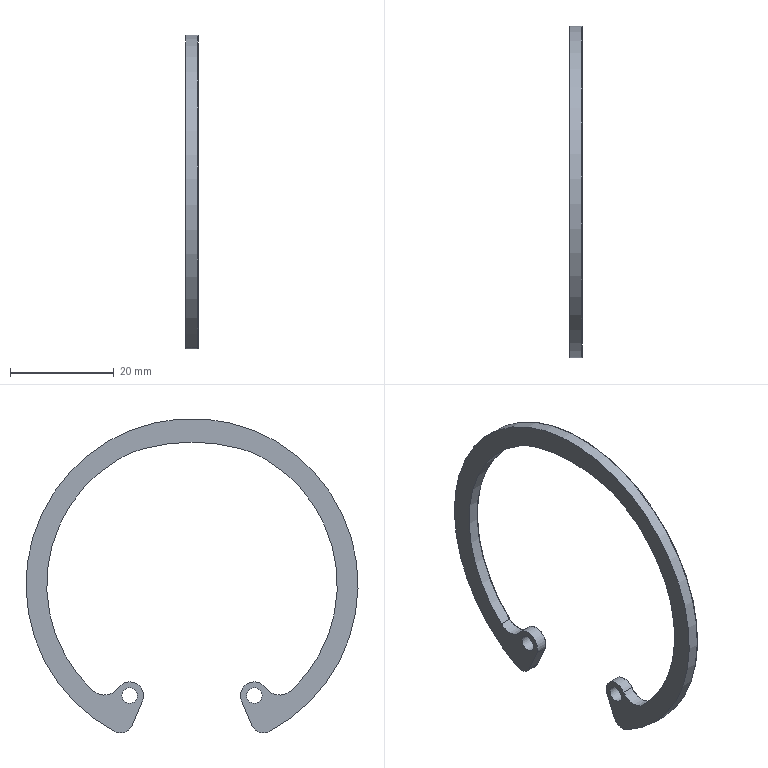Part | NX | features DATUM_CSYS 2, BLEND 1, EXTRUDE 1, SKETCH 1 | 1 solid | 36 faces | box 2.4 x 64 x 60.597 mm | volume 1716 mm3 | cylinder 18 | torus 12 | plane 6 | commonest cylinder face diameters 0.4 x4 3 x2 4.829 x2 5.31 x2 6.707 x2 40 x2
STEP:
#1=CARTESIAN_POINT('',(2.2,9.37,26.18));
#2=VERTEX_POINT('',#1);
#3=CARTESIAN_POINT('',(0.,9.37,26.18));
#4=VERTEX_POINT('',#3);
#5=CARTESIAN_POINT('',(2.4,9.37,26.18));
#6=DIRECTION('',(-1.,0.,0.));
#7=VECTOR('',#6,1000.);
#8=LINE('',#5,#7);
#9=EDGE_CURVE('',#2,#4,#8,.T.);
#10=ORIENTED_EDGE('',*,*,#9,.F.);
#11=CARTESIAN_POINT('',(2.2,-9.37,26.18));
#12=VERTEX_POINT('',#11);
#13=CARTESIAN_POINT('',(2.2,0.,-7.748));
#14=DIRECTION('',(-1.,0.,0.));
#15=DIRECTION('',(0.,0.,1.));
#16=AXIS2_PLACEMENT_3D('',#13,#14,#15);
#17=CIRCLE('',#16,35.198);
#18=EDGE_CURVE('',#2,#12,#17,.F.);
#19=ORIENTED_EDGE('',*,*,#18,.T.);
#20=CARTESIAN_POINT('',(0.,-9.37,26.18));
#21=VERTEX_POINT('',#20);
#22=CARTESIAN_POINT('',(2.4,-9.37,26.18));
#23=DIRECTION('',(-1.,0.,0.));
#24=VECTOR('',#23,1000.);
#25=LINE('',#22,#24);
#26=EDGE_CURVE('',#12,#21,#25,.T.);
#27=ORIENTED_EDGE('',*,*,#26,.T.);
#28=CARTESIAN_POINT('',(0.,0.,-7.748));
#29=DIRECTION('',(-1.,0.,0.));
#30=DIRECTION('',(0.,-1.,0.));
#31=AXIS2_PLACEMENT_3D('',#28,#29,#30);
#32=CIRCLE('',#31,35.198);
#33=EDGE_CURVE('',#21,#4,#32,.T.);
#34=ORIENTED_EDGE('',*,*,#33,.T.);
#35=EDGE_LOOP('',(#10,#19,#27,#34));
#36=FACE_BOUND('',#35,.T.);
#37=CARTESIAN_POINT('',(2.4,0.,-7.748));
#38=DIRECTION('',(-1.,0.,0.));
#39=DIRECTION('',(0.,0.,1.));
#40=AXIS2_PLACEMENT_3D('',#37,#38,#39);
#41=CYLINDRICAL_SURFACE('',#40,35.198);
#42=ADVANCED_FACE('',(#36),#41,.F.);
#43=CARTESIAN_POINT('',(2.2,14.16,24.156));
#44=VERTEX_POINT('',#43);
#45=CARTESIAN_POINT('',(0.,14.16,24.156));
#46=VERTEX_POINT('',#45);
#47=CARTESIAN_POINT('',(2.4,14.16,24.156));
#48=DIRECTION('',(-1.,0.,0.));
#49=VECTOR('',#48,1000.);
#50=LINE('',#47,#49);
#51=EDGE_CURVE('',#44,#46,#50,.T.);
#52=ORIENTED_EDGE('',*,*,#51,.F.);
#53=CARTESIAN_POINT('',(2.2,4.046,6.902));
#54=DIRECTION('',(-1.,0.,0.));
#55=DIRECTION('',(0.,0.,1.));
#56=AXIS2_PLACEMENT_3D('',#53,#54,#55);
#57=CIRCLE('',#56,20.);
#58=EDGE_CURVE('',#44,#2,#57,.F.);
#59=ORIENTED_EDGE('',*,*,#58,.T.);
#60=ORIENTED_EDGE('',*,*,#9,.T.);
#61=CARTESIAN_POINT('',(0.,4.046,6.902));
#62=DIRECTION('',(-1.,0.,0.));
#63=DIRECTION('',(0.,-1.,0.));
#64=AXIS2_PLACEMENT_3D('',#61,#62,#63);
#65=CIRCLE('',#64,20.);
#66=EDGE_CURVE('',#4,#46,#65,.T.);
#67=ORIENTED_EDGE('',*,*,#66,.T.);
#68=EDGE_LOOP('',(#52,#59,#60,#67));
#69=FACE_BOUND('',#68,.T.);
#70=CARTESIAN_POINT('',(2.4,4.046,6.902));
#71=DIRECTION('',(-1.,0.,0.));
#72=DIRECTION('',(0.,0.,1.));
#73=AXIS2_PLACEMENT_3D('',#70,#71,#72);
#74=CYLINDRICAL_SURFACE('',#73,20.);
#75=ADVANCED_FACE('',(#69),#74,.F.);
#76=CARTESIAN_POINT('',(2.2,19.208,-20.373));
#77=VERTEX_POINT('',#76);
#78=CARTESIAN_POINT('',(0.,19.208,-20.373));
#79=VERTEX_POINT('',#78);
#80=CARTESIAN_POINT('',(2.4,19.208,-20.373));
#81=DIRECTION('',(-1.,0.,0.));
#82=VECTOR('',#81,1000.);
#83=LINE('',#80,#82);
#84=EDGE_CURVE('',#77,#79,#83,.T.);
#85=ORIENTED_EDGE('',*,*,#84,.F.);
#86=CARTESIAN_POINT('',(2.2,0.,0.));
#87=DIRECTION('',(-1.,0.,0.));
#88=DIRECTION('',(0.,0.,1.));
#89=AXIS2_PLACEMENT_3D('',#86,#87,#88);
#90=CIRCLE('',#89,28.);
#91=EDGE_CURVE('',#77,#44,#90,.F.);
#92=ORIENTED_EDGE('',*,*,#91,.T.);
#93=ORIENTED_EDGE('',*,*,#51,.T.);
#94=CARTESIAN_POINT('',(0.,0.,0.));
#95=DIRECTION('',(-1.,0.,0.));
#96=DIRECTION('',(0.,-1.,0.));
#97=AXIS2_PLACEMENT_3D('',#94,#95,#96);
#98=CIRCLE('',#97,28.);
#99=EDGE_CURVE('',#46,#79,#98,.T.);
#100=ORIENTED_EDGE('',*,*,#99,.T.);
#101=EDGE_LOOP('',(#85,#92,#93,#100));
#102=FACE_BOUND('',#101,.T.);
#103=CARTESIAN_POINT('',(2.4,0.,0.));
#104=DIRECTION('',(-1.,0.,0.));
#105=DIRECTION('',(0.,0.,1.));
#106=AXIS2_PLACEMENT_3D('',#103,#104,#105);
#107=CYLINDRICAL_SURFACE('',#106,28.);
#108=ADVANCED_FACE('',(#102),#107,.F.);
#109=CARTESIAN_POINT('',(2.2,14.177,-19.88));
#110=VERTEX_POINT('',#109);
#111=CARTESIAN_POINT('',(0.,14.177,-19.88));
#112=VERTEX_POINT('',#111);
#113=CARTESIAN_POINT('',(2.4,14.177,-19.88));
#114=DIRECTION('',(-1.,0.,0.));
#115=VECTOR('',#114,1000.);
#116=LINE('',#113,#115);
#117=EDGE_CURVE('',#110,#112,#116,.T.);
#118=ORIENTED_EDGE('',*,*,#117,.F.);
#119=CARTESIAN_POINT('',(2.2,16.908,-17.932));
#120=DIRECTION('',(-1.,0.,0.));
#121=DIRECTION('',(0.,0.,1.));
#122=AXIS2_PLACEMENT_3D('',#119,#120,#121);
#123=CIRCLE('',#122,3.354);
#124=EDGE_CURVE('',#110,#77,#123,.F.);
#125=ORIENTED_EDGE('',*,*,#124,.T.);
#126=ORIENTED_EDGE('',*,*,#84,.T.);
#127=CARTESIAN_POINT('',(0.,16.908,-17.932));
#128=DIRECTION('',(-1.,0.,0.));
#129=DIRECTION('',(0.,-1.,0.));
#130=AXIS2_PLACEMENT_3D('',#127,#128,#129);
#131=CIRCLE('',#130,3.354);
#132=EDGE_CURVE('',#79,#112,#131,.T.);
#133=ORIENTED_EDGE('',*,*,#132,.T.);
#134=EDGE_LOOP('',(#118,#125,#126,#133));
#135=FACE_BOUND('',#134,.T.);
#136=CARTESIAN_POINT('',(2.4,16.908,-17.932));
#137=DIRECTION('',(-1.,0.,0.));
#138=DIRECTION('',(0.,0.,1.));
#139=AXIS2_PLACEMENT_3D('',#136,#137,#138);
#140=CYLINDRICAL_SURFACE('',#139,3.354);
#141=ADVANCED_FACE('',(#135),#140,.F.);
#142=CARTESIAN_POINT('',(2.2,14.162,-19.858));
#143=VERTEX_POINT('',#142);
#144=CARTESIAN_POINT('',(0.,14.162,-19.858));
#145=VERTEX_POINT('',#144);
#146=CARTESIAN_POINT('',(2.4,14.162,-19.858));
#147=DIRECTION('',(-1.,0.,0.));
#148=VECTOR('',#147,1000.);
#149=LINE('',#146,#148);
#150=EDGE_CURVE('',#143,#145,#149,.T.);
#151=ORIENTED_EDGE('',*,*,#150,.F.);
#152=CARTESIAN_POINT('',(2.2,14.177,-19.88));
#153=DIRECTION('',(0.,-0.5806,0.8142));
#154=VECTOR('',#153,1000.);
#155=LINE('',#152,#154);
#156=EDGE_CURVE('',#143,#110,#155,.F.);
#157=ORIENTED_EDGE('',*,*,#156,.T.);
#158=ORIENTED_EDGE('',*,*,#117,.T.);
#159=CARTESIAN_POINT('',(0.,14.177,-19.88));
#160=DIRECTION('',(0.,-0.5806,0.8142));
#161=VECTOR('',#160,1000.);
#162=LINE('',#159,#161);
#163=EDGE_CURVE('',#112,#145,#162,.T.);
#164=ORIENTED_EDGE('',*,*,#163,.T.);
#165=EDGE_LOOP('',(#151,#157,#158,#164));
#166=FACE_BOUND('',#165,.T.);
#167=CARTESIAN_POINT('',(2.4,14.177,-19.88));
#168=DIRECTION('',(0.,-0.8142,-0.5806));
#169=DIRECTION('',(0.,0.5806,-0.8142));
#170=AXIS2_PLACEMENT_3D('',#167,#168,#169);
#171=PLANE('',#170);
#172=ADVANCED_FACE('',(#166),#171,.F.);
#173=CARTESIAN_POINT('',(2.2,9.557,-22.44));
#174=VERTEX_POINT('',#173);
#175=CARTESIAN_POINT('',(0.,9.557,-22.44));
#176=VERTEX_POINT('',#175);
#177=CARTESIAN_POINT('',(2.4,9.557,-22.44));
#178=DIRECTION('',(-1.,0.,0.));
#179=VECTOR('',#178,1000.);
#180=LINE('',#177,#179);
#181=EDGE_CURVE('',#174,#176,#180,.T.);
#182=ORIENTED_EDGE('',*,*,#181,.F.);
#183=CARTESIAN_POINT('',(2.2,12.,-21.4));
#184=DIRECTION('',(-1.,0.,0.));
#185=DIRECTION('',(0.,0.,1.));
#186=AXIS2_PLACEMENT_3D('',#183,#184,#185);
#187=CIRCLE('',#186,2.655);
#188=EDGE_CURVE('',#174,#143,#187,.T.);
#189=ORIENTED_EDGE('',*,*,#188,.T.);
#190=ORIENTED_EDGE('',*,*,#150,.T.);
#191=CARTESIAN_POINT('',(0.,12.,-21.4));
#192=DIRECTION('',(1.,0.,0.));
#193=DIRECTION('',(0.,-1.,0.));
#194=AXIS2_PLACEMENT_3D('',#191,#192,#193);
#195=CIRCLE('',#194,2.655);
#196=EDGE_CURVE('',#145,#176,#195,.T.);
#197=ORIENTED_EDGE('',*,*,#196,.T.);
#198=EDGE_LOOP('',(#182,#189,#190,#197));
#199=FACE_BOUND('',#198,.T.);
#200=CARTESIAN_POINT('',(2.4,12.,-21.4));
#201=DIRECTION('',(-1.,0.,0.));
#202=DIRECTION('',(0.,0.,1.));
#203=AXIS2_PLACEMENT_3D('',#200,#201,#202);
#204=CYLINDRICAL_SURFACE('',#203,2.655);
#205=ADVANCED_FACE('',(#199),#204,.T.);
#206=CARTESIAN_POINT('',(2.2,11.554,-27.129));
#207=VERTEX_POINT('',#206);
#208=CARTESIAN_POINT('',(0.,11.554,-27.129));
#209=VERTEX_POINT('',#208);
#210=CARTESIAN_POINT('',(2.4,11.554,-27.129));
#211=DIRECTION('',(-1.,0.,0.));
#212=VECTOR('',#211,1000.);
#213=LINE('',#210,#212);
#214=EDGE_CURVE('',#207,#209,#213,.T.);
#215=ORIENTED_EDGE('',*,*,#214,.F.);
#216=CARTESIAN_POINT('',(2.2,9.557,-22.44));
#217=DIRECTION('',(0.,0.3918,-0.92));
#218=VECTOR('',#217,1000.);
#219=LINE('',#216,#218);
#220=EDGE_CURVE('',#207,#174,#219,.F.);
#221=ORIENTED_EDGE('',*,*,#220,.T.);
#222=ORIENTED_EDGE('',*,*,#181,.T.);
#223=CARTESIAN_POINT('',(0.,9.557,-22.44));
#224=DIRECTION('',(0.,0.3918,-0.92));
#225=VECTOR('',#224,1000.);
#226=LINE('',#223,#225);
#227=EDGE_CURVE('',#176,#209,#226,.T.);
#228=ORIENTED_EDGE('',*,*,#227,.T.);
#229=EDGE_LOOP('',(#215,#221,#222,#228));
#230=FACE_BOUND('',#229,.T.);
#231=CARTESIAN_POINT('',(2.4,9.557,-22.44));
#232=DIRECTION('',(0.,0.92,0.3918));
#233=DIRECTION('',(0.,-0.3918,0.92));
#234=AXIS2_PLACEMENT_3D('',#231,#232,#233);
#235=PLANE('',#234);
#236=ADVANCED_FACE('',(#230),#235,.F.);
#237=CARTESIAN_POINT('',(2.2,14.9,-28.319));
#238=VERTEX_POINT('',#237);
#239=CARTESIAN_POINT('',(0.,14.9,-28.319));
#240=VERTEX_POINT('',#239);
#241=CARTESIAN_POINT('',(2.4,14.9,-28.319));
#242=DIRECTION('',(-1.,0.,0.));
#243=VECTOR('',#242,1000.);
#244=LINE('',#241,#243);
#245=EDGE_CURVE('',#238,#240,#244,.T.);
#246=ORIENTED_EDGE('',*,*,#245,.F.);
#247=CARTESIAN_POINT('',(2.2,13.776,-26.183));
#248=DIRECTION('',(-1.,0.,0.));
#249=DIRECTION('',(0.,0.,1.));
#250=AXIS2_PLACEMENT_3D('',#247,#248,#249);
#251=CIRCLE('',#250,2.415);
#252=EDGE_CURVE('',#238,#207,#251,.T.);
#253=ORIENTED_EDGE('',*,*,#252,.T.);
#254=ORIENTED_EDGE('',*,*,#214,.T.);
#255=CARTESIAN_POINT('',(0.,13.776,-26.183));
#256=DIRECTION('',(1.,0.,0.));
#257=DIRECTION('',(0.,-1.,0.));
#258=AXIS2_PLACEMENT_3D('',#255,#256,#257);
#259=CIRCLE('',#258,2.415);
#260=EDGE_CURVE('',#209,#240,#259,.T.);
#261=ORIENTED_EDGE('',*,*,#260,.T.);
#262=EDGE_LOOP('',(#246,#253,#254,#261));
#263=FACE_BOUND('',#262,.T.);
#264=CARTESIAN_POINT('',(2.4,13.776,-26.183));
#265=DIRECTION('',(-1.,0.,0.));
#266=DIRECTION('',(0.,0.,1.));
#267=AXIS2_PLACEMENT_3D('',#264,#265,#266);
#268=CYLINDRICAL_SURFACE('',#267,2.415);
#269=ADVANCED_FACE('',(#263),#268,.T.);
#270=CARTESIAN_POINT('',(2.2,-14.9,-28.319));
#271=VERTEX_POINT('',#270);
#272=CARTESIAN_POINT('',(0.,-14.9,-28.319));
#273=VERTEX_POINT('',#272);
#274=CARTESIAN_POINT('',(2.4,-14.9,-28.319));
#275=DIRECTION('',(-1.,0.,0.));
#276=VECTOR('',#275,1000.);
#277=LINE('',#274,#276);
#278=EDGE_CURVE('',#271,#273,#277,.T.);
#279=ORIENTED_EDGE('',*,*,#278,.F.);
#280=CARTESIAN_POINT('',(2.2,0.,0.));
#281=DIRECTION('',(-1.,0.,0.));
#282=DIRECTION('',(0.,0.,1.));
#283=AXIS2_PLACEMENT_3D('',#280,#281,#282);
#284=CIRCLE('',#283,32.);
#285=EDGE_CURVE('',#271,#238,#284,.T.);
#286=ORIENTED_EDGE('',*,*,#285,.T.);
#287=ORIENTED_EDGE('',*,*,#245,.T.);
#288=CARTESIAN_POINT('',(0.,0.,0.));
#289=DIRECTION('',(1.,0.,0.));
#290=DIRECTION('',(0.,1.,0.));
#291=AXIS2_PLACEMENT_3D('',#288,#289,#290);
#292=CIRCLE('',#291,32.);
#293=EDGE_CURVE('',#240,#273,#292,.T.);
#294=ORIENTED_EDGE('',*,*,#293,.T.);
#295=EDGE_LOOP('',(#279,#286,#287,#294));
#296=FACE_BOUND('',#295,.T.);
#297=CARTESIAN_POINT('',(2.4,0.,0.));
#298=DIRECTION('',(-1.,0.,0.));
#299=DIRECTION('',(0.,0.,1.));
#300=AXIS2_PLACEMENT_3D('',#297,#298,#299);
#301=CYLINDRICAL_SURFACE('',#300,32.);
#302=ADVANCED_FACE('',(#296),#301,.T.);
#303=CARTESIAN_POINT('',(2.2,-11.554,-27.129));
#304=VERTEX_POINT('',#303);
#305=CARTESIAN_POINT('',(0.,-11.554,-27.129));
#306=VERTEX_POINT('',#305);
#307=CARTESIAN_POINT('',(2.4,-11.554,-27.129));
#308=DIRECTION('',(-1.,0.,0.));
#309=VECTOR('',#308,1000.);
#310=LINE('',#307,#309);
#311=EDGE_CURVE('',#304,#306,#310,.T.);
#312=ORIENTED_EDGE('',*,*,#311,.F.);
#313=CARTESIAN_POINT('',(2.2,-13.776,-26.183));
#314=DIRECTION('',(-1.,0.,0.));
#315=DIRECTION('',(0.,0.,1.));
#316=AXIS2_PLACEMENT_3D('',#313,#314,#315);
#317=CIRCLE('',#316,2.415);
#318=EDGE_CURVE('',#304,#271,#317,.T.);
#319=ORIENTED_EDGE('',*,*,#318,.T.);
#320=ORIENTED_EDGE('',*,*,#278,.T.);
#321=CARTESIAN_POINT('',(0.,-13.776,-26.183));
#322=DIRECTION('',(1.,0.,0.));
#323=DIRECTION('',(0.,1.,0.));
#324=AXIS2_PLACEMENT_3D('',#321,#322,#323);
#325=CIRCLE('',#324,2.415);
#326=EDGE_CURVE('',#273,#306,#325,.T.);
#327=ORIENTED_EDGE('',*,*,#326,.T.);
#328=EDGE_LOOP('',(#312,#319,#320,#327));
#329=FACE_BOUND('',#328,.T.);
#330=CARTESIAN_POINT('',(2.4,-13.776,-26.183));
#331=DIRECTION('',(-1.,0.,0.));
#332=DIRECTION('',(0.,0.,1.));
#333=AXIS2_PLACEMENT_3D('',#330,#331,#332);
#334=CYLINDRICAL_SURFACE('',#333,2.415);
#335=ADVANCED_FACE('',(#329),#334,.T.);
#336=CARTESIAN_POINT('',(2.2,-9.557,-22.44));
#337=VERTEX_POINT('',#336);
#338=CARTESIAN_POINT('',(0.,-9.557,-22.44));
#339=VERTEX_POINT('',#338);
#340=CARTESIAN_POINT('',(2.4,-9.557,-22.44));
#341=DIRECTION('',(-1.,0.,0.));
#342=VECTOR('',#341,1000.);
#343=LINE('',#340,#342);
#344=EDGE_CURVE('',#337,#339,#343,.T.);
#345=ORIENTED_EDGE('',*,*,#344,.F.);
#346=CARTESIAN_POINT('',(2.2,-11.554,-27.129));
#347=DIRECTION('',(0.,0.3918,0.92));
#348=VECTOR('',#347,1000.);
#349=LINE('',#346,#348);
#350=EDGE_CURVE('',#337,#304,#349,.F.);
#351=ORIENTED_EDGE('',*,*,#350,.T.);
#352=ORIENTED_EDGE('',*,*,#311,.T.);
#353=CARTESIAN_POINT('',(0.,-11.554,-27.129));
#354=DIRECTION('',(0.,0.3918,0.92));
#355=VECTOR('',#354,1000.);
#356=LINE('',#353,#355);
#357=EDGE_CURVE('',#306,#339,#356,.T.);
#358=ORIENTED_EDGE('',*,*,#357,.T.);
#359=EDGE_LOOP('',(#345,#351,#352,#358));
#360=FACE_BOUND('',#359,.T.);
#361=CARTESIAN_POINT('',(2.4,-11.554,-27.129));
#362=DIRECTION('',(0.,-0.92,0.3918));
#363=DIRECTION('',(0.,-0.3918,-0.92));
#364=AXIS2_PLACEMENT_3D('',#361,#362,#363);
#365=PLANE('',#364);
#366=ADVANCED_FACE('',(#360),#365,.F.);
#367=CARTESIAN_POINT('',(2.2,-14.162,-19.858));
#368=VERTEX_POINT('',#367);
#369=CARTESIAN_POINT('',(0.,-14.162,-19.858));
#370=VERTEX_POINT('',#369);
#371=CARTESIAN_POINT('',(2.4,-14.162,-19.858));
#372=DIRECTION('',(-1.,0.,0.));
#373=VECTOR('',#372,1000.);
#374=LINE('',#371,#373);
#375=EDGE_CURVE('',#368,#370,#374,.T.);
#376=ORIENTED_EDGE('',*,*,#375,.F.);
#377=CARTESIAN_POINT('',(2.2,-12.,-21.4));
#378=DIRECTION('',(-1.,0.,0.));
#379=DIRECTION('',(0.,0.,1.));
#380=AXIS2_PLACEMENT_3D('',#377,#378,#379);
#381=CIRCLE('',#380,2.655);
#382=EDGE_CURVE('',#368,#337,#381,.T.);
#383=ORIENTED_EDGE('',*,*,#382,.T.);
#384=ORIENTED_EDGE('',*,*,#344,.T.);
#385=CARTESIAN_POINT('',(0.,-12.,-21.4));
#386=DIRECTION('',(1.,0.,0.));
#387=DIRECTION('',(0.,1.,0.));
#388=AXIS2_PLACEMENT_3D('',#385,#386,#387);
#389=CIRCLE('',#388,2.655);
#390=EDGE_CURVE('',#339,#370,#389,.T.);
#391=ORIENTED_EDGE('',*,*,#390,.T.);
#392=EDGE_LOOP('',(#376,#383,#384,#391));
#393=FACE_BOUND('',#392,.T.);
#394=CARTESIAN_POINT('',(2.4,-12.,-21.4));
#395=DIRECTION('',(-1.,0.,0.));
#396=DIRECTION('',(0.,0.,1.));
#397=AXIS2_PLACEMENT_3D('',#394,#395,#396);
#398=CYLINDRICAL_SURFACE('',#397,2.655);
#399=ADVANCED_FACE('',(#393),#398,.T.);
#400=CARTESIAN_POINT('',(2.2,-14.177,-19.88));
#401=VERTEX_POINT('',#400);
#402=CARTESIAN_POINT('',(0.,-14.177,-19.88));
#403=VERTEX_POINT('',#402);
#404=CARTESIAN_POINT('',(2.4,-14.177,-19.88));
#405=DIRECTION('',(-1.,0.,0.));
#406=VECTOR('',#405,1000.);
#407=LINE('',#404,#406);
#408=EDGE_CURVE('',#401,#403,#407,.T.);
#409=ORIENTED_EDGE('',*,*,#408,.F.);
#410=CARTESIAN_POINT('',(2.2,-14.162,-19.858));
#411=DIRECTION('',(0.,-0.5806,-0.8142));
#412=VECTOR('',#411,1000.);
#413=LINE('',#410,#412);
#414=EDGE_CURVE('',#401,#368,#413,.F.);
#415=ORIENTED_EDGE('',*,*,#414,.T.);
#416=ORIENTED_EDGE('',*,*,#375,.T.);
#417=CARTESIAN_POINT('',(0.,-14.162,-19.858));
#418=DIRECTION('',(0.,-0.5806,-0.8142));
#419=VECTOR('',#418,1000.);
#420=LINE('',#417,#419);
#421=EDGE_CURVE('',#370,#403,#420,.T.);
#422=ORIENTED_EDGE('',*,*,#421,.T.);
#423=EDGE_LOOP('',(#409,#415,#416,#422));
#424=FACE_BOUND('',#423,.T.);
#425=CARTESIAN_POINT('',(2.4,-14.162,-19.858));
#426=DIRECTION('',(0.,0.8142,-0.5806));
#427=DIRECTION('',(0.,0.5806,0.8142));
#428=AXIS2_PLACEMENT_3D('',#425,#426,#427);
#429=PLANE('',#428);
#430=ADVANCED_FACE('',(#424),#429,.F.);
#431=CARTESIAN_POINT('',(2.2,-19.208,-20.373));
#432=VERTEX_POINT('',#431);
#433=CARTESIAN_POINT('',(0.,-19.208,-20.373));
#434=VERTEX_POINT('',#433);
#435=CARTESIAN_POINT('',(2.4,-19.208,-20.373));
#436=DIRECTION('',(-1.,0.,0.));
#437=VECTOR('',#436,1000.);
#438=LINE('',#435,#437);
#439=EDGE_CURVE('',#432,#434,#438,.T.);
#440=ORIENTED_EDGE('',*,*,#439,.F.);
#441=CARTESIAN_POINT('',(2.2,-16.908,-17.932));
#442=DIRECTION('',(-1.,0.,0.));
#443=DIRECTION('',(0.,0.,1.));
#444=AXIS2_PLACEMENT_3D('',#441,#442,#443);
#445=CIRCLE('',#444,3.354);
#446=EDGE_CURVE('',#432,#401,#445,.F.);
#447=ORIENTED_EDGE('',*,*,#446,.T.);
#448=ORIENTED_EDGE('',*,*,#408,.T.);
#449=CARTESIAN_POINT('',(0.,-16.908,-17.932));
#450=DIRECTION('',(-1.,0.,0.));
#451=DIRECTION('',(0.,1.,0.));
#452=AXIS2_PLACEMENT_3D('',#449,#450,#451);
#453=CIRCLE('',#452,3.354);
#454=EDGE_CURVE('',#403,#434,#453,.T.);
#455=ORIENTED_EDGE('',*,*,#454,.T.);
#456=EDGE_LOOP('',(#440,#447,#448,#455));
#457=FACE_BOUND('',#456,.T.);
#458=CARTESIAN_POINT('',(2.4,-16.908,-17.932));
#459=DIRECTION('',(-1.,0.,0.));
#460=DIRECTION('',(0.,0.,1.));
#461=AXIS2_PLACEMENT_3D('',#458,#459,#460);
#462=CYLINDRICAL_SURFACE('',#461,3.354);
#463=ADVANCED_FACE('',(#457),#462,.F.);
#464=CARTESIAN_POINT('',(2.2,-14.16,24.156));
#465=VERTEX_POINT('',#464);
#466=CARTESIAN_POINT('',(0.,-14.16,24.156));
#467=VERTEX_POINT('',#466);
#468=CARTESIAN_POINT('',(2.4,-14.16,24.156));
#469=DIRECTION('',(-1.,0.,0.));
#470=VECTOR('',#469,1000.);
#471=LINE('',#468,#470);
#472=EDGE_CURVE('',#465,#467,#471,.T.);
#473=ORIENTED_EDGE('',*,*,#472,.F.);
#474=CARTESIAN_POINT('',(2.2,0.,0.));
#475=DIRECTION('',(-1.,0.,0.));
#476=DIRECTION('',(0.,0.,1.));
#477=AXIS2_PLACEMENT_3D('',#474,#475,#476);
#478=CIRCLE('',#477,28.);
#479=EDGE_CURVE('',#465,#432,#478,.F.);
#480=ORIENTED_EDGE('',*,*,#479,.T.);
#481=ORIENTED_EDGE('',*,*,#439,.T.);
#482=CARTESIAN_POINT('',(0.,0.,0.));
#483=DIRECTION('',(-1.,0.,0.));
#484=DIRECTION('',(0.,1.,0.));
#485=AXIS2_PLACEMENT_3D('',#482,#483,#484);
#486=CIRCLE('',#485,28.);
#487=EDGE_CURVE('',#434,#467,#486,.T.);
#488=ORIENTED_EDGE('',*,*,#487,.T.);
#489=EDGE_LOOP('',(#473,#480,#481,#488));
#490=FACE_BOUND('',#489,.T.);
#491=CARTESIAN_POINT('',(2.4,0.,0.));
#492=DIRECTION('',(-1.,0.,0.));
#493=DIRECTION('',(0.,0.,1.));
#494=AXIS2_PLACEMENT_3D('',#491,#492,#493);
#495=CYLINDRICAL_SURFACE('',#494,28.);
#496=ADVANCED_FACE('',(#490),#495,.F.);
#497=CARTESIAN_POINT('',(2.4,10.5,-21.4));
#498=VERTEX_POINT('',#497);
#499=CARTESIAN_POINT('',(2.4,12.,-21.4));
#500=DIRECTION('',(-1.,0.,0.));
#501=DIRECTION('',(0.,-1.,0.));
#502=AXIS2_PLACEMENT_3D('',#499,#500,#501);
#503=CIRCLE('',#502,1.5);
#504=EDGE_CURVE('',#498,#498,#503,.T.);
#505=ORIENTED_EDGE('',*,*,#504,.F.);
#506=EDGE_LOOP('',(#505));
#507=FACE_BOUND('',#506,.T.);
#508=CARTESIAN_POINT('',(0.,10.5,-21.4));
#509=VERTEX_POINT('',#508);
#510=CARTESIAN_POINT('',(0.,12.,-21.4));
#511=DIRECTION('',(-1.,0.,0.));
#512=DIRECTION('',(0.,-1.,0.));
#513=AXIS2_PLACEMENT_3D('',#510,#511,#512);
#514=CIRCLE('',#513,1.5);
#515=EDGE_CURVE('',#509,#509,#514,.T.);
#516=ORIENTED_EDGE('',*,*,#515,.T.);
#517=EDGE_LOOP('',(#516));
#518=FACE_BOUND('',#517,.T.);
#519=CARTESIAN_POINT('',(2.4,12.,-21.4));
#520=DIRECTION('',(-1.,0.,0.));
#521=DIRECTION('',(0.,0.,1.));
#522=AXIS2_PLACEMENT_3D('',#519,#520,#521);
#523=CYLINDRICAL_SURFACE('',#522,1.5);
#524=ADVANCED_FACE('',(#507,#518),#523,.F.);
#525=ORIENTED_EDGE('',*,*,#26,.F.);
#526=CARTESIAN_POINT('',(2.2,-4.046,6.902));
#527=DIRECTION('',(-1.,0.,0.));
#528=DIRECTION('',(0.,0.,1.));
#529=AXIS2_PLACEMENT_3D('',#526,#527,#528);
#530=CIRCLE('',#529,20.);
#531=EDGE_CURVE('',#12,#465,#530,.F.);
#532=ORIENTED_EDGE('',*,*,#531,.T.);
#533=ORIENTED_EDGE('',*,*,#472,.T.);
#534=CARTESIAN_POINT('',(0.,-4.046,6.902));
#535=DIRECTION('',(-1.,0.,0.));
#536=DIRECTION('',(0.,1.,0.));
#537=AXIS2_PLACEMENT_3D('',#534,#535,#536);
#538=CIRCLE('',#537,20.);
#539=EDGE_CURVE('',#467,#21,#538,.T.);
#540=ORIENTED_EDGE('',*,*,#539,.T.);
#541=EDGE_LOOP('',(#525,#532,#533,#540));
#542=FACE_BOUND('',#541,.T.);
#543=CARTESIAN_POINT('',(2.4,-4.046,6.902));
#544=DIRECTION('',(-1.,0.,0.));
#545=DIRECTION('',(0.,0.,1.));
#546=AXIS2_PLACEMENT_3D('',#543,#544,#545);
#547=CYLINDRICAL_SURFACE('',#546,20.);
#548=ADVANCED_FACE('',(#542),#547,.F.);
#549=CARTESIAN_POINT('',(2.4,-10.5,-21.4));
#550=VERTEX_POINT('',#549);
#551=CARTESIAN_POINT('',(2.4,-12.,-21.4));
#552=DIRECTION('',(1.,0.,0.));
#553=DIRECTION('',(0.,1.,0.));
#554=AXIS2_PLACEMENT_3D('',#551,#552,#553);
#555=CIRCLE('',#554,1.5);
#556=EDGE_CURVE('',#550,#550,#555,.T.);
#557=ORIENTED_EDGE('',*,*,#556,.T.);
#558=EDGE_LOOP('',(#557));
#559=FACE_BOUND('',#558,.T.);
#560=CARTESIAN_POINT('',(0.,-10.5,-21.4));
#561=VERTEX_POINT('',#560);
#562=CARTESIAN_POINT('',(0.,-12.,-21.4));
#563=DIRECTION('',(1.,0.,0.));
#564=DIRECTION('',(0.,1.,0.));
#565=AXIS2_PLACEMENT_3D('',#562,#563,#564);
#566=CIRCLE('',#565,1.5);
#567=EDGE_CURVE('',#561,#561,#566,.T.);
#568=ORIENTED_EDGE('',*,*,#567,.F.);
#569=EDGE_LOOP('',(#568));
#570=FACE_BOUND('',#569,.T.);
#571=CARTESIAN_POINT('',(2.4,-12.,-21.4));
#572=DIRECTION('',(-1.,0.,0.));
#573=DIRECTION('',(0.,0.,1.));
#574=AXIS2_PLACEMENT_3D('',#571,#572,#573);
#575=CYLINDRICAL_SURFACE('',#574,1.5);
#576=ADVANCED_FACE('',(#559,#570),#575,.F.);
#577=CARTESIAN_POINT('',(2.4,19.345,-20.518));
#578=VERTEX_POINT('',#577);
#579=CARTESIAN_POINT('',(2.4,14.014,-19.996));
#580=VERTEX_POINT('',#579);
#581=CARTESIAN_POINT('',(2.4,16.908,-17.932));
#582=DIRECTION('',(-1.,0.,0.));
#583=DIRECTION('',(0.,0.,1.));
#584=AXIS2_PLACEMENT_3D('',#581,#582,#583);
#585=CIRCLE('',#584,3.554);
#586=EDGE_CURVE('',#578,#580,#585,.T.);
#587=ORIENTED_EDGE('',*,*,#586,.T.);
#588=CARTESIAN_POINT('',(2.4,13.999,-19.974));
#589=VERTEX_POINT('',#588);
#590=CARTESIAN_POINT('',(2.4,3.5,-5.252));
#591=DIRECTION('',(0.,-0.5806,0.8142));
#592=VECTOR('',#591,1000.);
#593=LINE('',#590,#592);
#594=EDGE_CURVE('',#580,#589,#593,.T.);
#595=ORIENTED_EDGE('',*,*,#594,.T.);
#596=CARTESIAN_POINT('',(2.4,9.741,-22.362));
#597=VERTEX_POINT('',#596);
#598=CARTESIAN_POINT('',(2.4,12.,-21.4));
#599=DIRECTION('',(-1.,0.,0.));
#600=DIRECTION('',(0.,0.,1.));
#601=AXIS2_PLACEMENT_3D('',#598,#599,#600);
#602=CIRCLE('',#601,2.455);
#603=EDGE_CURVE('',#589,#597,#602,.F.);
#604=ORIENTED_EDGE('',*,*,#603,.T.);
#605=CARTESIAN_POINT('',(2.4,11.738,-27.05));
#606=VERTEX_POINT('',#605);
#607=CARTESIAN_POINT('',(2.4,2.977,-6.48));
#608=DIRECTION('',(0.,0.3918,-0.92));
#609=VECTOR('',#608,1000.);
#610=LINE('',#607,#609);
#611=EDGE_CURVE('',#597,#606,#610,.T.);
#612=ORIENTED_EDGE('',*,*,#611,.T.);
#613=CARTESIAN_POINT('',(2.4,14.807,-28.142));
#614=VERTEX_POINT('',#613);
#615=CARTESIAN_POINT('',(2.4,13.776,-26.183));
#616=DIRECTION('',(-1.,0.,0.));
#617=DIRECTION('',(0.,0.,1.));
#618=AXIS2_PLACEMENT_3D('',#615,#616,#617);
#619=CIRCLE('',#618,2.215);
#620=EDGE_CURVE('',#606,#614,#619,.F.);
#621=ORIENTED_EDGE('',*,*,#620,.T.);
#622=CARTESIAN_POINT('',(2.4,-14.807,-28.142));
#623=VERTEX_POINT('',#622);
#624=CARTESIAN_POINT('',(2.4,0.,0.));
#625=DIRECTION('',(-1.,0.,0.));
#626=DIRECTION('',(0.,0.,1.));
#627=AXIS2_PLACEMENT_3D('',#624,#625,#626);
#628=CIRCLE('',#627,31.8);
#629=EDGE_CURVE('',#614,#623,#628,.F.);
#630=ORIENTED_EDGE('',*,*,#629,.T.);
#631=CARTESIAN_POINT('',(2.4,-11.738,-27.05));
#632=VERTEX_POINT('',#631);
#633=CARTESIAN_POINT('',(2.4,-13.776,-26.183));
#634=DIRECTION('',(-1.,0.,0.));
#635=DIRECTION('',(0.,0.,1.));
#636=AXIS2_PLACEMENT_3D('',#633,#634,#635);
#637=CIRCLE('',#636,2.215);
#638=EDGE_CURVE('',#623,#632,#637,.F.);
#639=ORIENTED_EDGE('',*,*,#638,.T.);
#640=CARTESIAN_POINT('',(2.4,-9.741,-22.362));
#641=VERTEX_POINT('',#640);
#642=CARTESIAN_POINT('',(2.4,-2.977,-6.48));
#643=DIRECTION('',(0.,0.3918,0.92));
#644=VECTOR('',#643,1000.);
#645=LINE('',#642,#644);
#646=EDGE_CURVE('',#632,#641,#645,.T.);
#647=ORIENTED_EDGE('',*,*,#646,.T.);
#648=CARTESIAN_POINT('',(2.4,-13.999,-19.974));
#649=VERTEX_POINT('',#648);
#650=CARTESIAN_POINT('',(2.4,-12.,-21.4));
#651=DIRECTION('',(-1.,0.,0.));
#652=DIRECTION('',(0.,0.,1.));
#653=AXIS2_PLACEMENT_3D('',#650,#651,#652);
#654=CIRCLE('',#653,2.455);
#655=EDGE_CURVE('',#641,#649,#654,.F.);
#656=ORIENTED_EDGE('',*,*,#655,.T.);
#657=CARTESIAN_POINT('',(2.4,-14.014,-19.996));
#658=VERTEX_POINT('',#657);
#659=CARTESIAN_POINT('',(2.4,-3.5,-5.252));
#660=DIRECTION('',(0.,-0.5806,-0.8142));
#661=VECTOR('',#660,1000.);
#662=LINE('',#659,#661);
#663=EDGE_CURVE('',#649,#658,#662,.T.);
#664=ORIENTED_EDGE('',*,*,#663,.T.);
#665=CARTESIAN_POINT('',(2.4,-19.345,-20.518));
#666=VERTEX_POINT('',#665);
#667=CARTESIAN_POINT('',(2.4,-16.908,-17.932));
#668=DIRECTION('',(-1.,0.,0.));
#669=DIRECTION('',(0.,0.,1.));
#670=AXIS2_PLACEMENT_3D('',#667,#668,#669);
#671=CIRCLE('',#670,3.554);
#672=EDGE_CURVE('',#658,#666,#671,.T.);
#673=ORIENTED_EDGE('',*,*,#672,.T.);
#674=CARTESIAN_POINT('',(2.4,-14.261,24.328));
#675=VERTEX_POINT('',#674);
#676=CARTESIAN_POINT('',(2.4,0.,0.));
#677=DIRECTION('',(-1.,0.,0.));
#678=DIRECTION('',(0.,0.,1.));
#679=AXIS2_PLACEMENT_3D('',#676,#677,#678);
#680=CIRCLE('',#679,28.2);
#681=EDGE_CURVE('',#666,#675,#680,.T.);
#682=ORIENTED_EDGE('',*,*,#681,.T.);
#683=CARTESIAN_POINT('',(2.4,-9.423,26.373));
#684=VERTEX_POINT('',#683);
#685=CARTESIAN_POINT('',(2.4,-4.046,6.902));
#686=DIRECTION('',(-1.,0.,0.));
#687=DIRECTION('',(0.,0.,1.));
#688=AXIS2_PLACEMENT_3D('',#685,#686,#687);
#689=CIRCLE('',#688,20.2);
#690=EDGE_CURVE('',#675,#684,#689,.T.);
#691=ORIENTED_EDGE('',*,*,#690,.T.);
#692=CARTESIAN_POINT('',(2.4,9.423,26.373));
#693=VERTEX_POINT('',#692);
#694=CARTESIAN_POINT('',(2.4,0.,-7.748));
#695=DIRECTION('',(-1.,0.,0.));
#696=DIRECTION('',(0.,0.,1.));
#697=AXIS2_PLACEMENT_3D('',#694,#695,#696);
#698=CIRCLE('',#697,35.398);
#699=EDGE_CURVE('',#684,#693,#698,.T.);
#700=ORIENTED_EDGE('',*,*,#699,.T.);
#701=CARTESIAN_POINT('',(2.4,14.261,24.328));
#702=VERTEX_POINT('',#701);
#703=CARTESIAN_POINT('',(2.4,4.046,6.902));
#704=DIRECTION('',(-1.,0.,0.));
#705=DIRECTION('',(0.,0.,1.));
#706=AXIS2_PLACEMENT_3D('',#703,#704,#705);
#707=CIRCLE('',#706,20.2);
#708=EDGE_CURVE('',#693,#702,#707,.T.);
#709=ORIENTED_EDGE('',*,*,#708,.T.);
#710=CARTESIAN_POINT('',(2.4,0.,0.));
#711=DIRECTION('',(-1.,0.,0.));
#712=DIRECTION('',(0.,0.,1.));
#713=AXIS2_PLACEMENT_3D('',#710,#711,#712);
#714=CIRCLE('',#713,28.2);
#715=EDGE_CURVE('',#702,#578,#714,.T.);
#716=ORIENTED_EDGE('',*,*,#715,.T.);
#717=EDGE_LOOP('',(#587,#595,#604,#612,#621,#630,#639,#647,#656,#664,#673,#682,#691,#700,#709,#716));
#718=FACE_BOUND('',#717,.T.);
#719=ORIENTED_EDGE('',*,*,#504,.T.);
#720=EDGE_LOOP('',(#719));
#721=FACE_BOUND('',#720,.T.);
#722=ORIENTED_EDGE('',*,*,#556,.F.);
#723=EDGE_LOOP('',(#722));
#724=FACE_BOUND('',#723,.T.);
#725=CARTESIAN_POINT('',(2.4,0.,-7.748));
#726=DIRECTION('',(-1.,0.,0.));
#727=DIRECTION('',(0.,0.,1.));
#728=AXIS2_PLACEMENT_3D('',#725,#726,#727);
#729=PLANE('',#728);
#730=ADVANCED_FACE('',(#718,#721,#724),#729,.F.);
#731=ORIENTED_EDGE('',*,*,#33,.F.);
#732=ORIENTED_EDGE('',*,*,#539,.F.);
#733=ORIENTED_EDGE('',*,*,#487,.F.);
#734=ORIENTED_EDGE('',*,*,#454,.F.);
#735=ORIENTED_EDGE('',*,*,#421,.F.);
#736=ORIENTED_EDGE('',*,*,#390,.F.);
#737=ORIENTED_EDGE('',*,*,#357,.F.);
#738=ORIENTED_EDGE('',*,*,#326,.F.);
#739=ORIENTED_EDGE('',*,*,#293,.F.);
#740=ORIENTED_EDGE('',*,*,#260,.F.);
#741=ORIENTED_EDGE('',*,*,#227,.F.);
#742=ORIENTED_EDGE('',*,*,#196,.F.);
#743=ORIENTED_EDGE('',*,*,#163,.F.);
#744=ORIENTED_EDGE('',*,*,#132,.F.);
#745=ORIENTED_EDGE('',*,*,#99,.F.);
#746=ORIENTED_EDGE('',*,*,#66,.F.);
#747=EDGE_LOOP('',(#731,#732,#733,#734,#735,#736,#737,#738,#739,#740,#741,#742,#743,#744,#745,#746));
#748=FACE_BOUND('',#747,.T.);
#749=ORIENTED_EDGE('',*,*,#515,.F.);
#750=EDGE_LOOP('',(#749));
#751=FACE_BOUND('',#750,.T.);
#752=ORIENTED_EDGE('',*,*,#567,.T.);
#753=EDGE_LOOP('',(#752));
#754=FACE_BOUND('',#753,.T.);
#755=CARTESIAN_POINT('',(0.,0.,-7.748));
#756=DIRECTION('',(-1.,0.,0.));
#757=DIRECTION('',(0.,0.,1.));
#758=AXIS2_PLACEMENT_3D('',#755,#756,#757);
#759=PLANE('',#758);
#760=ADVANCED_FACE('',(#748,#751,#754),#759,.T.);
#761=CARTESIAN_POINT('',(2.2,-14.261,24.328));
#762=DIRECTION('',(0.,-0.8627,-0.5057));
#763=DIRECTION('',(0.,0.5057,-0.8627));
#764=AXIS2_PLACEMENT_3D('',#761,#762,#763);
#765=CIRCLE('',#764,0.2);
#766=EDGE_CURVE('',#465,#675,#765,.T.);
#767=ORIENTED_EDGE('',*,*,#766,.F.);
#768=ORIENTED_EDGE('',*,*,#531,.F.);
#769=CARTESIAN_POINT('',(2.2,-9.423,26.373));
#770=DIRECTION('',(0.,0.9639,0.2662));
#771=DIRECTION('',(0.,-0.2662,0.9639));
#772=AXIS2_PLACEMENT_3D('',#769,#770,#771);
#773=CIRCLE('',#772,0.2);
#774=EDGE_CURVE('',#684,#12,#773,.T.);
#775=ORIENTED_EDGE('',*,*,#774,.F.);
#776=ORIENTED_EDGE('',*,*,#690,.F.);
#777=EDGE_LOOP('',(#767,#768,#775,#776));
#778=FACE_BOUND('',#777,.T.);
#779=CARTESIAN_POINT('',(2.2,-4.046,6.902));
#780=DIRECTION('',(-1.,0.,0.));
#781=DIRECTION('',(0.,0.,1.));
#782=AXIS2_PLACEMENT_3D('',#779,#780,#781);
#783=TOROIDAL_SURFACE('',#782,20.2,0.2);
#784=ADVANCED_FACE('',(#778),#783,.T.);
#785=ORIENTED_EDGE('',*,*,#774,.T.);
#786=ORIENTED_EDGE('',*,*,#18,.F.);
#787=CARTESIAN_POINT('',(2.2,9.423,26.373));
#788=DIRECTION('',(0.,0.9639,-0.2662));
#789=DIRECTION('',(0.,0.2662,0.9639));
#790=AXIS2_PLACEMENT_3D('',#787,#788,#789);
#791=CIRCLE('',#790,0.2);
#792=EDGE_CURVE('',#693,#2,#791,.T.);
#793=ORIENTED_EDGE('',*,*,#792,.F.);
#794=ORIENTED_EDGE('',*,*,#699,.F.);
#795=EDGE_LOOP('',(#785,#786,#793,#794));
#796=FACE_BOUND('',#795,.T.);
#797=CARTESIAN_POINT('',(2.2,0.,-7.748));
#798=DIRECTION('',(-1.,0.,0.));
#799=DIRECTION('',(0.,0.,1.));
#800=AXIS2_PLACEMENT_3D('',#797,#798,#799);
#801=TOROIDAL_SURFACE('',#800,35.398,0.2);
#802=ADVANCED_FACE('',(#796),#801,.T.);
#803=ORIENTED_EDGE('',*,*,#766,.T.);
#804=ORIENTED_EDGE('',*,*,#681,.F.);
#805=CARTESIAN_POINT('',(2.2,-19.345,-20.518));
#806=DIRECTION('',(0.,0.7276,-0.686));
#807=DIRECTION('',(0.,0.686,0.7276));
#808=AXIS2_PLACEMENT_3D('',#805,#806,#807);
#809=CIRCLE('',#808,0.2);
#810=EDGE_CURVE('',#432,#666,#809,.T.);
#811=ORIENTED_EDGE('',*,*,#810,.F.);
#812=ORIENTED_EDGE('',*,*,#479,.F.);
#813=EDGE_LOOP('',(#803,#804,#811,#812));
#814=FACE_BOUND('',#813,.T.);
#815=CARTESIAN_POINT('',(2.2,0.,0.));
#816=DIRECTION('',(-1.,0.,0.));
#817=DIRECTION('',(0.,0.,1.));
#818=AXIS2_PLACEMENT_3D('',#815,#816,#817);
#819=TOROIDAL_SURFACE('',#818,28.2,0.2);
#820=ADVANCED_FACE('',(#814),#819,.T.);
#821=ORIENTED_EDGE('',*,*,#792,.T.);
#822=ORIENTED_EDGE('',*,*,#58,.F.);
#823=CARTESIAN_POINT('',(2.2,14.261,24.328));
#824=DIRECTION('',(0.,0.8627,-0.5057));
#825=DIRECTION('',(0.,0.5057,0.8627));
#826=AXIS2_PLACEMENT_3D('',#823,#824,#825);
#827=CIRCLE('',#826,0.2);
#828=EDGE_CURVE('',#702,#44,#827,.T.);
#829=ORIENTED_EDGE('',*,*,#828,.F.);
#830=ORIENTED_EDGE('',*,*,#708,.F.);
#831=EDGE_LOOP('',(#821,#822,#829,#830));
#832=FACE_BOUND('',#831,.T.);
#833=CARTESIAN_POINT('',(2.2,4.046,6.902));
#834=DIRECTION('',(-1.,0.,0.));
#835=DIRECTION('',(0.,0.,1.));
#836=AXIS2_PLACEMENT_3D('',#833,#834,#835);
#837=TOROIDAL_SURFACE('',#836,20.2,0.2);
#838=ADVANCED_FACE('',(#832),#837,.T.);
#839=ORIENTED_EDGE('',*,*,#810,.T.);
#840=ORIENTED_EDGE('',*,*,#672,.F.);
#841=CARTESIAN_POINT('',(2.2,-14.014,-19.996));
#842=DIRECTION('',(0.,0.5806,0.8142));
#843=DIRECTION('',(0.,-0.8142,0.5806));
#844=AXIS2_PLACEMENT_3D('',#841,#842,#843);
#845=CIRCLE('',#844,0.2);
#846=EDGE_CURVE('',#401,#658,#845,.T.);
#847=ORIENTED_EDGE('',*,*,#846,.F.);
#848=ORIENTED_EDGE('',*,*,#446,.F.);
#849=EDGE_LOOP('',(#839,#840,#847,#848));
#850=FACE_BOUND('',#849,.T.);
#851=CARTESIAN_POINT('',(2.2,-16.908,-17.932));
#852=DIRECTION('',(-1.,0.,0.));
#853=DIRECTION('',(0.,0.,1.));
#854=AXIS2_PLACEMENT_3D('',#851,#852,#853);
#855=TOROIDAL_SURFACE('',#854,3.554,0.2);
#856=ADVANCED_FACE('',(#850),#855,.T.);
#857=ORIENTED_EDGE('',*,*,#828,.T.);
#858=ORIENTED_EDGE('',*,*,#91,.F.);
#859=CARTESIAN_POINT('',(2.2,19.345,-20.518));
#860=DIRECTION('',(0.,-0.7276,-0.686));
#861=DIRECTION('',(0.,0.686,-0.7276));
#862=AXIS2_PLACEMENT_3D('',#859,#860,#861);
#863=CIRCLE('',#862,0.2);
#864=EDGE_CURVE('',#578,#77,#863,.T.);
#865=ORIENTED_EDGE('',*,*,#864,.F.);
#866=ORIENTED_EDGE('',*,*,#715,.F.);
#867=EDGE_LOOP('',(#857,#858,#865,#866));
#868=FACE_BOUND('',#867,.T.);
#869=CARTESIAN_POINT('',(2.2,0.,0.));
#870=DIRECTION('',(-1.,0.,0.));
#871=DIRECTION('',(0.,0.,1.));
#872=AXIS2_PLACEMENT_3D('',#869,#870,#871);
#873=TOROIDAL_SURFACE('',#872,28.2,0.2);
#874=ADVANCED_FACE('',(#868),#873,.T.);
#875=ORIENTED_EDGE('',*,*,#846,.T.);
#876=ORIENTED_EDGE('',*,*,#663,.F.);
#877=CARTESIAN_POINT('',(2.2,-13.999,-19.974));
#878=DIRECTION('',(0.,0.5806,0.8142));
#879=DIRECTION('',(0.,-0.8142,0.5806));
#880=AXIS2_PLACEMENT_3D('',#877,#878,#879);
#881=CIRCLE('',#880,0.2);
#882=EDGE_CURVE('',#368,#649,#881,.T.);
#883=ORIENTED_EDGE('',*,*,#882,.F.);
#884=ORIENTED_EDGE('',*,*,#414,.F.);
#885=EDGE_LOOP('',(#875,#876,#883,#884));
#886=FACE_BOUND('',#885,.T.);
#887=CARTESIAN_POINT('',(2.2,-3.5,-5.252));
#888=DIRECTION('',(0.,-0.5806,-0.8142));
#889=DIRECTION('',(0.,0.8142,-0.5806));
#890=AXIS2_PLACEMENT_3D('',#887,#888,#889);
#891=CYLINDRICAL_SURFACE('',#890,0.2);
#892=ADVANCED_FACE('',(#886),#891,.T.);
#893=ORIENTED_EDGE('',*,*,#864,.T.);
#894=ORIENTED_EDGE('',*,*,#124,.F.);
#895=CARTESIAN_POINT('',(2.2,14.014,-19.996));
#896=DIRECTION('',(0.,-0.5806,0.8142));
#897=DIRECTION('',(0.,-0.8142,-0.5806));
#898=AXIS2_PLACEMENT_3D('',#895,#896,#897);
#899=CIRCLE('',#898,0.2);
#900=EDGE_CURVE('',#580,#110,#899,.T.);
#901=ORIENTED_EDGE('',*,*,#900,.F.);
#902=ORIENTED_EDGE('',*,*,#586,.F.);
#903=EDGE_LOOP('',(#893,#894,#901,#902));
#904=FACE_BOUND('',#903,.T.);
#905=CARTESIAN_POINT('',(2.2,16.908,-17.932));
#906=DIRECTION('',(-1.,0.,0.));
#907=DIRECTION('',(0.,0.,1.));
#908=AXIS2_PLACEMENT_3D('',#905,#906,#907);
#909=TOROIDAL_SURFACE('',#908,3.554,0.2);
#910=ADVANCED_FACE('',(#904),#909,.T.);
#911=ORIENTED_EDGE('',*,*,#882,.T.);
#912=ORIENTED_EDGE('',*,*,#655,.F.);
#913=CARTESIAN_POINT('',(2.2,-9.741,-22.362));
#914=DIRECTION('',(0.,-0.3918,-0.92));
#915=DIRECTION('',(0.,0.92,-0.3918));
#916=AXIS2_PLACEMENT_3D('',#913,#914,#915);
#917=CIRCLE('',#916,0.2);
#918=EDGE_CURVE('',#337,#641,#917,.T.);
#919=ORIENTED_EDGE('',*,*,#918,.F.);
#920=ORIENTED_EDGE('',*,*,#382,.F.);
#921=EDGE_LOOP('',(#911,#912,#919,#920));
#922=FACE_BOUND('',#921,.T.);
#923=CARTESIAN_POINT('',(2.2,-12.,-21.4));
#924=DIRECTION('',(-1.,0.,0.));
#925=DIRECTION('',(0.,0.,1.));
#926=AXIS2_PLACEMENT_3D('',#923,#924,#925);
#927=TOROIDAL_SURFACE('',#926,2.455,0.2);
#928=ADVANCED_FACE('',(#922),#927,.T.);
#929=ORIENTED_EDGE('',*,*,#900,.T.);
#930=ORIENTED_EDGE('',*,*,#156,.F.);
#931=CARTESIAN_POINT('',(2.2,13.999,-19.974));
#932=DIRECTION('',(0.,-0.5806,0.8142));
#933=DIRECTION('',(0.,-0.8142,-0.5806));
#934=AXIS2_PLACEMENT_3D('',#931,#932,#933);
#935=CIRCLE('',#934,0.2);
#936=EDGE_CURVE('',#589,#143,#935,.T.);
#937=ORIENTED_EDGE('',*,*,#936,.F.);
#938=ORIENTED_EDGE('',*,*,#594,.F.);
#939=EDGE_LOOP('',(#929,#930,#937,#938));
#940=FACE_BOUND('',#939,.T.);
#941=CARTESIAN_POINT('',(2.2,3.5,-5.252));
#942=DIRECTION('',(0.,-0.5806,0.8142));
#943=DIRECTION('',(0.,-0.8142,-0.5806));
#944=AXIS2_PLACEMENT_3D('',#941,#942,#943);
#945=CYLINDRICAL_SURFACE('',#944,0.2);
#946=ADVANCED_FACE('',(#940),#945,.T.);
#947=ORIENTED_EDGE('',*,*,#918,.T.);
#948=ORIENTED_EDGE('',*,*,#646,.F.);
#949=CARTESIAN_POINT('',(2.2,-11.738,-27.05));
#950=DIRECTION('',(0.,-0.3918,-0.92));
#951=DIRECTION('',(0.,0.92,-0.3918));
#952=AXIS2_PLACEMENT_3D('',#949,#950,#951);
#953=CIRCLE('',#952,0.2);
#954=EDGE_CURVE('',#304,#632,#953,.T.);
#955=ORIENTED_EDGE('',*,*,#954,.F.);
#956=ORIENTED_EDGE('',*,*,#350,.F.);
#957=EDGE_LOOP('',(#947,#948,#955,#956));
#958=FACE_BOUND('',#957,.T.);
#959=CARTESIAN_POINT('',(2.2,-2.977,-6.48));
#960=DIRECTION('',(0.,0.3918,0.92));
#961=DIRECTION('',(0.,-0.92,0.3918));
#962=AXIS2_PLACEMENT_3D('',#959,#960,#961);
#963=CYLINDRICAL_SURFACE('',#962,0.2);
#964=ADVANCED_FACE('',(#958),#963,.T.);
#965=ORIENTED_EDGE('',*,*,#936,.T.);
#966=ORIENTED_EDGE('',*,*,#188,.F.);
#967=CARTESIAN_POINT('',(2.2,9.741,-22.362));
#968=DIRECTION('',(0.,0.3918,-0.92));
#969=DIRECTION('',(0.,0.92,0.3918));
#970=AXIS2_PLACEMENT_3D('',#967,#968,#969);
#971=CIRCLE('',#970,0.2);
#972=EDGE_CURVE('',#597,#174,#971,.T.);
#973=ORIENTED_EDGE('',*,*,#972,.F.);
#974=ORIENTED_EDGE('',*,*,#603,.F.);
#975=EDGE_LOOP('',(#965,#966,#973,#974));
#976=FACE_BOUND('',#975,.T.);
#977=CARTESIAN_POINT('',(2.2,12.,-21.4));
#978=DIRECTION('',(-1.,0.,0.));
#979=DIRECTION('',(0.,0.,1.));
#980=AXIS2_PLACEMENT_3D('',#977,#978,#979);
#981=TOROIDAL_SURFACE('',#980,2.455,0.2);
#982=ADVANCED_FACE('',(#976),#981,.T.);
#983=ORIENTED_EDGE('',*,*,#954,.T.);
#984=ORIENTED_EDGE('',*,*,#638,.F.);
#985=CARTESIAN_POINT('',(2.2,-14.807,-28.142));
#986=DIRECTION('',(0.,-0.885,0.4656));
#987=DIRECTION('',(0.,-0.4656,-0.885));
#988=AXIS2_PLACEMENT_3D('',#985,#986,#987);
#989=CIRCLE('',#988,0.2);
#990=EDGE_CURVE('',#271,#623,#989,.T.);
#991=ORIENTED_EDGE('',*,*,#990,.F.);
#992=ORIENTED_EDGE('',*,*,#318,.F.);
#993=EDGE_LOOP('',(#983,#984,#991,#992));
#994=FACE_BOUND('',#993,.T.);
#995=CARTESIAN_POINT('',(2.2,-13.776,-26.183));
#996=DIRECTION('',(-1.,0.,0.));
#997=DIRECTION('',(0.,0.,1.));
#998=AXIS2_PLACEMENT_3D('',#995,#996,#997);
#999=TOROIDAL_SURFACE('',#998,2.215,0.2);
#1000=ADVANCED_FACE('',(#994),#999,.T.);
#1001=ORIENTED_EDGE('',*,*,#972,.T.);
#1002=ORIENTED_EDGE('',*,*,#220,.F.);
#1003=CARTESIAN_POINT('',(2.2,11.738,-27.05));
#1004=DIRECTION('',(0.,0.3918,-0.92));
#1005=DIRECTION('',(0.,0.92,0.3918));
#1006=AXIS2_PLACEMENT_3D('',#1003,#1004,#1005);
#1007=CIRCLE('',#1006,0.2);
#1008=EDGE_CURVE('',#606,#207,#1007,.T.);
#1009=ORIENTED_EDGE('',*,*,#1008,.F.);
#1010=ORIENTED_EDGE('',*,*,#611,.F.);
#1011=EDGE_LOOP('',(#1001,#1002,#1009,#1010));
#1012=FACE_BOUND('',#1011,.T.);
#1013=CARTESIAN_POINT('',(2.2,2.977,-6.48));
#1014=DIRECTION('',(0.,0.3918,-0.92));
#1015=DIRECTION('',(0.,0.92,0.3918));
#1016=AXIS2_PLACEMENT_3D('',#1013,#1014,#1015);
#1017=CYLINDRICAL_SURFACE('',#1016,0.2);
#1018=ADVANCED_FACE('',(#1012),#1017,.T.);
#1019=ORIENTED_EDGE('',*,*,#990,.T.);
#1020=ORIENTED_EDGE('',*,*,#629,.F.);
#1021=CARTESIAN_POINT('',(2.2,14.807,-28.142));
#1022=DIRECTION('',(0.,-0.885,-0.4656));
#1023=DIRECTION('',(0.,0.4656,-0.885));
#1024=AXIS2_PLACEMENT_3D('',#1021,#1022,#1023);
#1025=CIRCLE('',#1024,0.2);
#1026=EDGE_CURVE('',#238,#614,#1025,.T.);
#1027=ORIENTED_EDGE('',*,*,#1026,.F.);
#1028=ORIENTED_EDGE('',*,*,#285,.F.);
#1029=EDGE_LOOP('',(#1019,#1020,#1027,#1028));
#1030=FACE_BOUND('',#1029,.T.);
#1031=CARTESIAN_POINT('',(2.2,0.,0.));
#1032=DIRECTION('',(-1.,0.,0.));
#1033=DIRECTION('',(0.,0.,1.));
#1034=AXIS2_PLACEMENT_3D('',#1031,#1032,#1033);
#1035=TOROIDAL_SURFACE('',#1034,31.8,0.2);
#1036=ADVANCED_FACE('',(#1030),#1035,.T.);
#1037=ORIENTED_EDGE('',*,*,#1008,.T.);
#1038=ORIENTED_EDGE('',*,*,#252,.F.);
#1039=ORIENTED_EDGE('',*,*,#1026,.T.);
#1040=ORIENTED_EDGE('',*,*,#620,.F.);
#1041=EDGE_LOOP('',(#1037,#1038,#1039,#1040));
#1042=FACE_BOUND('',#1041,.T.);
#1043=CARTESIAN_POINT('',(2.2,13.776,-26.183));
#1044=DIRECTION('',(-1.,0.,0.));
#1045=DIRECTION('',(0.,0.,1.));
#1046=AXIS2_PLACEMENT_3D('',#1043,#1044,#1045);
#1047=TOROIDAL_SURFACE('',#1046,2.215,0.2);
#1048=ADVANCED_FACE('',(#1042),#1047,.T.);
#1049=CLOSED_SHELL('',(#42,#75,#108,#141,#172,#205,#236,#269,#302,#335,#366,#399,#430,#463,#496,#524,#548,#576,#730,#760,#784,#802,#820,#838,#856,#874,#892,#910,#928,#946,#964,#982,#1000,#1018,#1036,#1048));
#1050=MANIFOLD_SOLID_BREP('',#1049);
#1051=(LENGTH_UNIT()NAMED_UNIT(*)SI_UNIT(.MILLI.,.METRE.));
#1052=UNCERTAINTY_MEASURE_WITH_UNIT(LENGTH_MEASURE(0.00001),#1051,'','');
#1053=(NAMED_UNIT(*)PLANE_ANGLE_UNIT()SI_UNIT($,.RADIAN.));
#1054=(NAMED_UNIT(*)SI_UNIT($,.STERADIAN.)SOLID_ANGLE_UNIT());
#1055=(GEOMETRIC_REPRESENTATION_CONTEXT(3)GLOBAL_UNCERTAINTY_ASSIGNED_CONTEXT((#1052))GLOBAL_UNIT_ASSIGNED_CONTEXT((#1051,#1053,#1054))REPRESENTATION_CONTEXT('',''));
#1056=ADVANCED_BREP_SHAPE_REPRESENTATION('',(#1050),#1055);